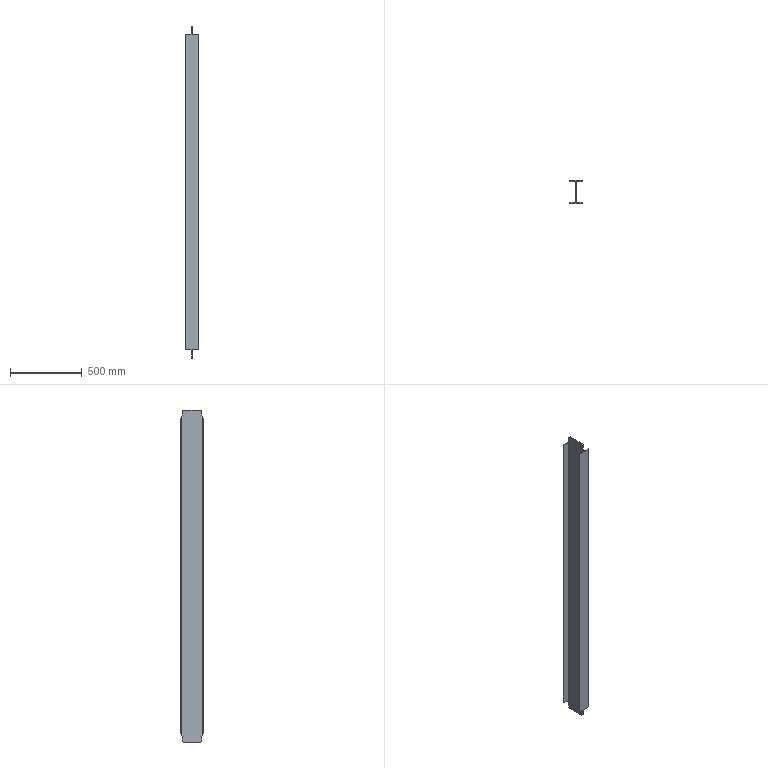Part | SolidWorks | features Chamfer 1, Extrusion 1, ICE 1 | 1 solid | 26 faces | box 88 x 160 x 2320 mm | volume 4382373 mm3 | plane 26
STEP:
#1=CARTESIAN_POINT('',(44.,-80.,1103.));
#2=VERTEX_POINT('',#1);
#3=CARTESIAN_POINT('',(44.,-80.,-1103.));
#4=VERTEX_POINT('',#3);
#5=CARTESIAN_POINT('',(44.,-80.,1160.));
#6=DIRECTION('',(0.,0.,-1.));
#7=VECTOR('',#6,1000.);
#8=LINE('',#5,#7);
#9=EDGE_CURVE('',#2,#4,#8,.T.);
#10=ORIENTED_EDGE('',*,*,#9,.F.);
#11=CARTESIAN_POINT('',(-44.,-80.,1103.));
#12=VERTEX_POINT('',#11);
#13=CARTESIAN_POINT('',(-44.,-80.,1103.));
#14=DIRECTION('',(1.,0.,0.));
#15=VECTOR('',#14,1000.);
#16=LINE('',#13,#15);
#17=EDGE_CURVE('',#12,#2,#16,.T.);
#18=ORIENTED_EDGE('',*,*,#17,.F.);
#19=CARTESIAN_POINT('',(-44.,-80.,-1103.));
#20=VERTEX_POINT('',#19);
#21=CARTESIAN_POINT('',(-44.,-80.,1160.));
#22=DIRECTION('',(0.,0.,-1.));
#23=VECTOR('',#22,1000.);
#24=LINE('',#21,#23);
#25=EDGE_CURVE('',#12,#20,#24,.T.);
#26=ORIENTED_EDGE('',*,*,#25,.T.);
#27=CARTESIAN_POINT('',(-44.,-80.,-1103.));
#28=DIRECTION('',(1.,0.,0.));
#29=VECTOR('',#28,1000.);
#30=LINE('',#27,#29);
#31=EDGE_CURVE('',#20,#4,#30,.T.);
#32=ORIENTED_EDGE('',*,*,#31,.T.);
#33=EDGE_LOOP('',(#10,#18,#26,#32));
#34=FACE_OUTER_BOUND('',#33,.T.);
#35=CARTESIAN_POINT('',(44.,-80.,1160.));
#36=DIRECTION('',(0.,1.,0.));
#37=DIRECTION('',(-1.,0.,0.));
#38=AXIS2_PLACEMENT_3D('',#35,#36,#37);
#39=PLANE('',#38);
#40=ADVANCED_FACE('',(#34),#39,.F.);
#41=CARTESIAN_POINT('',(44.,-76.,1103.));
#42=VERTEX_POINT('',#41);
#43=CARTESIAN_POINT('',(44.,-76.,-1103.));
#44=VERTEX_POINT('',#43);
#45=CARTESIAN_POINT('',(44.,-76.,1160.));
#46=DIRECTION('',(0.,0.,-1.));
#47=VECTOR('',#46,1000.);
#48=LINE('',#45,#47);
#49=EDGE_CURVE('',#42,#44,#48,.T.);
#50=ORIENTED_EDGE('',*,*,#49,.F.);
#51=CARTESIAN_POINT('',(44.,-72.,1103.));
#52=DIRECTION('',(0.,1.,0.));
#53=VECTOR('',#52,1000.);
#54=LINE('',#51,#53);
#55=EDGE_CURVE('',#2,#42,#54,.T.);
#56=ORIENTED_EDGE('',*,*,#55,.F.);
#57=ORIENTED_EDGE('',*,*,#9,.T.);
#58=CARTESIAN_POINT('',(44.,-72.,-1103.));
#59=DIRECTION('',(0.,-1.,0.));
#60=VECTOR('',#59,1000.);
#61=LINE('',#58,#60);
#62=EDGE_CURVE('',#44,#4,#61,.T.);
#63=ORIENTED_EDGE('',*,*,#62,.F.);
#64=EDGE_LOOP('',(#50,#56,#57,#63));
#65=FACE_OUTER_BOUND('',#64,.T.);
#66=CARTESIAN_POINT('',(44.,-80.,1160.));
#67=DIRECTION('',(-1.,0.,0.));
#68=DIRECTION('',(0.,-1.,0.));
#69=AXIS2_PLACEMENT_3D('',#66,#67,#68);
#70=PLANE('',#69);
#71=ADVANCED_FACE('',(#65),#70,.F.);
#72=CARTESIAN_POINT('',(3.,-72.,1103.));
#73=VERTEX_POINT('',#72);
#74=CARTESIAN_POINT('',(3.,-72.,-1103.));
#75=VERTEX_POINT('',#74);
#76=CARTESIAN_POINT('',(3.,-72.,1160.));
#77=DIRECTION('',(0.,0.,-1.));
#78=VECTOR('',#77,1000.);
#79=LINE('',#76,#78);
#80=EDGE_CURVE('',#73,#75,#79,.T.);
#81=ORIENTED_EDGE('',*,*,#80,.F.);
#82=CARTESIAN_POINT('',(44.,-76.,1103.));
#83=DIRECTION('',(0.9953,-0.0971,0.));
#84=VECTOR('',#83,1000.);
#85=LINE('',#82,#84);
#86=EDGE_CURVE('',#73,#42,#85,.T.);
#87=ORIENTED_EDGE('',*,*,#86,.T.);
#88=ORIENTED_EDGE('',*,*,#49,.T.);
#89=CARTESIAN_POINT('',(44.,-76.,-1103.));
#90=DIRECTION('',(-0.9953,0.0971,0.));
#91=VECTOR('',#90,1000.);
#92=LINE('',#89,#91);
#93=EDGE_CURVE('',#44,#75,#92,.T.);
#94=ORIENTED_EDGE('',*,*,#93,.T.);
#95=EDGE_LOOP('',(#81,#87,#88,#94));
#96=FACE_OUTER_BOUND('',#95,.T.);
#97=CARTESIAN_POINT('',(44.,-76.,1160.));
#98=DIRECTION('',(-0.0971,-0.9953,0.));
#99=DIRECTION('',(0.9953,-0.0971,0.));
#100=AXIS2_PLACEMENT_3D('',#97,#98,#99);
#101=PLANE('',#100);
#102=ADVANCED_FACE('',(#96),#101,.F.);
#103=CARTESIAN_POINT('',(3.,-66.706,-1153.294));
#104=VERTEX_POINT('',#103);
#105=CARTESIAN_POINT('',(3.,-306.022,1120.208));
#106=DIRECTION('',(0.,0.1047,-0.9945));
#107=VECTOR('',#106,1000.);
#108=LINE('',#105,#107);
#109=EDGE_CURVE('',#75,#104,#108,.T.);
#110=ORIENTED_EDGE('',*,*,#109,.T.);
#111=CARTESIAN_POINT('',(3.,-60.,-1160.));
#112=VERTEX_POINT('',#111);
#113=CARTESIAN_POINT('',(3.,-66.706,-1153.294));
#114=DIRECTION('',(0.,0.7071,-0.7071));
#115=VECTOR('',#114,1000.);
#116=LINE('',#113,#115);
#117=EDGE_CURVE('',#104,#112,#116,.T.);
#118=ORIENTED_EDGE('',*,*,#117,.T.);
#119=CARTESIAN_POINT('',(3.,60.,-1160.));
#120=VERTEX_POINT('',#119);
#121=CARTESIAN_POINT('',(3.,72.,-1160.));
#122=DIRECTION('',(0.,1.,0.));
#123=VECTOR('',#122,1000.);
#124=LINE('',#121,#123);
#125=EDGE_CURVE('',#112,#120,#124,.T.);
#126=ORIENTED_EDGE('',*,*,#125,.T.);
#127=CARTESIAN_POINT('',(3.,66.706,-1153.294));
#128=VERTEX_POINT('',#127);
#129=CARTESIAN_POINT('',(3.,66.706,-1153.294));
#130=DIRECTION('',(0.,0.7071,0.7071));
#131=VECTOR('',#130,1000.);
#132=LINE('',#129,#131);
#133=EDGE_CURVE('',#120,#128,#132,.T.);
#134=ORIENTED_EDGE('',*,*,#133,.T.);
#135=CARTESIAN_POINT('',(3.,72.,-1103.));
#136=VERTEX_POINT('',#135);
#137=CARTESIAN_POINT('',(3.,307.6,1135.2));
#138=DIRECTION('',(0.,0.1047,0.9945));
#139=VECTOR('',#138,1000.);
#140=LINE('',#137,#139);
#141=EDGE_CURVE('',#128,#136,#140,.T.);
#142=ORIENTED_EDGE('',*,*,#141,.T.);
#143=CARTESIAN_POINT('',(3.,72.,1103.));
#144=VERTEX_POINT('',#143);
#145=CARTESIAN_POINT('',(3.,72.,1160.));
#146=DIRECTION('',(0.,0.,-1.));
#147=VECTOR('',#146,1000.);
#148=LINE('',#145,#147);
#149=EDGE_CURVE('',#144,#136,#148,.T.);
#150=ORIENTED_EDGE('',*,*,#149,.F.);
#151=CARTESIAN_POINT('',(3.,66.628,1154.033));
#152=VERTEX_POINT('',#151);
#153=CARTESIAN_POINT('',(3.,66.066,1159.375));
#154=DIRECTION('',(0.,-0.1047,0.9945));
#155=VECTOR('',#154,1000.);
#156=LINE('',#153,#155);
#157=EDGE_CURVE('',#144,#152,#156,.T.);
#158=ORIENTED_EDGE('',*,*,#157,.T.);
#159=CARTESIAN_POINT('',(3.,59.257,1160.));
#160=VERTEX_POINT('',#159);
#161=CARTESIAN_POINT('',(3.,59.257,1160.));
#162=DIRECTION('',(0.,-0.7772,0.6292));
#163=VECTOR('',#162,1000.);
#164=LINE('',#161,#163);
#165=EDGE_CURVE('',#152,#160,#164,.T.);
#166=ORIENTED_EDGE('',*,*,#165,.T.);
#167=CARTESIAN_POINT('',(3.,-59.257,1160.));
#168=VERTEX_POINT('',#167);
#169=CARTESIAN_POINT('',(3.,72.,1160.));
#170=DIRECTION('',(0.,1.,0.));
#171=VECTOR('',#170,1000.);
#172=LINE('',#169,#171);
#173=EDGE_CURVE('',#168,#160,#172,.T.);
#174=ORIENTED_EDGE('',*,*,#173,.F.);
#175=CARTESIAN_POINT('',(3.,-66.628,1154.033));
#176=VERTEX_POINT('',#175);
#177=CARTESIAN_POINT('',(3.,-59.257,1160.));
#178=DIRECTION('',(0.,-0.7772,-0.6292));
#179=VECTOR('',#178,1000.);
#180=LINE('',#177,#179);
#181=EDGE_CURVE('',#168,#176,#180,.T.);
#182=ORIENTED_EDGE('',*,*,#181,.T.);
#183=CARTESIAN_POINT('',(3.,-64.488,1174.367));
#184=DIRECTION('',(0.,-0.1047,-0.9945));
#185=VECTOR('',#184,1000.);
#186=LINE('',#183,#185);
#187=EDGE_CURVE('',#176,#73,#186,.T.);
#188=ORIENTED_EDGE('',*,*,#187,.T.);
#189=ORIENTED_EDGE('',*,*,#80,.T.);
#190=EDGE_LOOP('',(#110,#118,#126,#134,#142,#150,#158,#166,#174,#182,#188,#189));
#191=FACE_OUTER_BOUND('',#190,.T.);
#192=CARTESIAN_POINT('',(3.,72.,1160.));
#193=DIRECTION('',(-1.,0.,0.));
#194=DIRECTION('',(0.,0.,1.));
#195=AXIS2_PLACEMENT_3D('',#192,#193,#194);
#196=PLANE('',#195);
#197=ADVANCED_FACE('',(#191),#196,.F.);
#198=ORIENTED_EDGE('',*,*,#149,.T.);
#199=CARTESIAN_POINT('',(44.,76.,-1103.));
#200=VERTEX_POINT('',#199);
#201=CARTESIAN_POINT('',(44.,76.,-1103.));
#202=DIRECTION('',(0.9953,0.0971,0.));
#203=VECTOR('',#202,1000.);
#204=LINE('',#201,#203);
#205=EDGE_CURVE('',#136,#200,#204,.T.);
#206=ORIENTED_EDGE('',*,*,#205,.T.);
#207=CARTESIAN_POINT('',(44.,76.,1103.));
#208=VERTEX_POINT('',#207);
#209=CARTESIAN_POINT('',(44.,76.,1160.));
#210=DIRECTION('',(0.,0.,-1.));
#211=VECTOR('',#210,1000.);
#212=LINE('',#209,#211);
#213=EDGE_CURVE('',#208,#200,#212,.T.);
#214=ORIENTED_EDGE('',*,*,#213,.F.);
#215=CARTESIAN_POINT('',(44.,76.,1103.));
#216=DIRECTION('',(-0.9953,-0.0971,0.));
#217=VECTOR('',#216,1000.);
#218=LINE('',#215,#217);
#219=EDGE_CURVE('',#208,#144,#218,.T.);
#220=ORIENTED_EDGE('',*,*,#219,.T.);
#221=EDGE_LOOP('',(#198,#206,#214,#220));
#222=FACE_OUTER_BOUND('',#221,.T.);
#223=CARTESIAN_POINT('',(44.,76.,1160.));
#224=DIRECTION('',(-0.0971,0.9953,0.));
#225=DIRECTION('',(-0.9953,-0.0971,0.));
#226=AXIS2_PLACEMENT_3D('',#223,#224,#225);
#227=PLANE('',#226);
#228=ADVANCED_FACE('',(#222),#227,.F.);
#229=ORIENTED_EDGE('',*,*,#213,.T.);
#230=CARTESIAN_POINT('',(44.,80.,-1103.));
#231=VERTEX_POINT('',#230);
#232=CARTESIAN_POINT('',(44.,72.,-1103.));
#233=DIRECTION('',(0.,-1.,0.));
#234=VECTOR('',#233,1000.);
#235=LINE('',#232,#234);
#236=EDGE_CURVE('',#231,#200,#235,.T.);
#237=ORIENTED_EDGE('',*,*,#236,.F.);
#238=CARTESIAN_POINT('',(44.,80.,1103.));
#239=VERTEX_POINT('',#238);
#240=CARTESIAN_POINT('',(44.,80.,1160.));
#241=DIRECTION('',(0.,0.,-1.));
#242=VECTOR('',#241,1000.);
#243=LINE('',#240,#242);
#244=EDGE_CURVE('',#239,#231,#243,.T.);
#245=ORIENTED_EDGE('',*,*,#244,.F.);
#246=CARTESIAN_POINT('',(44.,72.,1103.));
#247=DIRECTION('',(0.,1.,0.));
#248=VECTOR('',#247,1000.);
#249=LINE('',#246,#248);
#250=EDGE_CURVE('',#208,#239,#249,.T.);
#251=ORIENTED_EDGE('',*,*,#250,.F.);
#252=EDGE_LOOP('',(#229,#237,#245,#251));
#253=FACE_OUTER_BOUND('',#252,.T.);
#254=CARTESIAN_POINT('',(44.,80.,1160.));
#255=DIRECTION('',(-1.,0.,0.));
#256=DIRECTION('',(0.,0.,1.));
#257=AXIS2_PLACEMENT_3D('',#254,#255,#256);
#258=PLANE('',#257);
#259=ADVANCED_FACE('',(#253),#258,.F.);
#260=ORIENTED_EDGE('',*,*,#244,.T.);
#261=CARTESIAN_POINT('',(-44.,80.,-1103.));
#262=VERTEX_POINT('',#261);
#263=CARTESIAN_POINT('',(-44.,80.,-1103.));
#264=DIRECTION('',(1.,0.,0.));
#265=VECTOR('',#264,1000.);
#266=LINE('',#263,#265);
#267=EDGE_CURVE('',#262,#231,#266,.T.);
#268=ORIENTED_EDGE('',*,*,#267,.F.);
#269=CARTESIAN_POINT('',(-44.,80.,1103.));
#270=VERTEX_POINT('',#269);
#271=CARTESIAN_POINT('',(-44.,80.,1160.));
#272=DIRECTION('',(0.,0.,-1.));
#273=VECTOR('',#272,1000.);
#274=LINE('',#271,#273);
#275=EDGE_CURVE('',#270,#262,#274,.T.);
#276=ORIENTED_EDGE('',*,*,#275,.F.);
#277=CARTESIAN_POINT('',(-44.,80.,1103.));
#278=DIRECTION('',(1.,0.,0.));
#279=VECTOR('',#278,1000.);
#280=LINE('',#277,#279);
#281=EDGE_CURVE('',#270,#239,#280,.T.);
#282=ORIENTED_EDGE('',*,*,#281,.T.);
#283=EDGE_LOOP('',(#260,#268,#276,#282));
#284=FACE_OUTER_BOUND('',#283,.T.);
#285=CARTESIAN_POINT('',(44.,80.,1160.));
#286=DIRECTION('',(0.,-1.,0.));
#287=DIRECTION('',(1.,0.,0.));
#288=AXIS2_PLACEMENT_3D('',#285,#286,#287);
#289=PLANE('',#288);
#290=ADVANCED_FACE('',(#284),#289,.F.);
#291=ORIENTED_EDGE('',*,*,#275,.T.);
#292=CARTESIAN_POINT('',(-44.,76.,-1103.));
#293=VERTEX_POINT('',#292);
#294=CARTESIAN_POINT('',(-44.,72.,-1103.));
#295=DIRECTION('',(0.,-1.,0.));
#296=VECTOR('',#295,1000.);
#297=LINE('',#294,#296);
#298=EDGE_CURVE('',#262,#293,#297,.T.);
#299=ORIENTED_EDGE('',*,*,#298,.T.);
#300=CARTESIAN_POINT('',(-44.,76.,1103.));
#301=VERTEX_POINT('',#300);
#302=CARTESIAN_POINT('',(-44.,76.,1160.));
#303=DIRECTION('',(0.,0.,-1.));
#304=VECTOR('',#303,1000.);
#305=LINE('',#302,#304);
#306=EDGE_CURVE('',#301,#293,#305,.T.);
#307=ORIENTED_EDGE('',*,*,#306,.F.);
#308=CARTESIAN_POINT('',(-44.,72.,1103.));
#309=DIRECTION('',(0.,1.,0.));
#310=VECTOR('',#309,1000.);
#311=LINE('',#308,#310);
#312=EDGE_CURVE('',#301,#270,#311,.T.);
#313=ORIENTED_EDGE('',*,*,#312,.T.);
#314=EDGE_LOOP('',(#291,#299,#307,#313));
#315=FACE_OUTER_BOUND('',#314,.T.);
#316=CARTESIAN_POINT('',(-44.,80.,1160.));
#317=DIRECTION('',(1.,0.,0.));
#318=DIRECTION('',(0.,1.,0.));
#319=AXIS2_PLACEMENT_3D('',#316,#317,#318);
#320=PLANE('',#319);
#321=ADVANCED_FACE('',(#315),#320,.F.);
#322=ORIENTED_EDGE('',*,*,#306,.T.);
#323=CARTESIAN_POINT('',(-3.,72.,-1103.));
#324=VERTEX_POINT('',#323);
#325=CARTESIAN_POINT('',(-44.,76.,-1103.));
#326=DIRECTION('',(0.9953,-0.0971,0.));
#327=VECTOR('',#326,1000.);
#328=LINE('',#325,#327);
#329=EDGE_CURVE('',#293,#324,#328,.T.);
#330=ORIENTED_EDGE('',*,*,#329,.T.);
#331=CARTESIAN_POINT('',(-3.,72.,1103.));
#332=VERTEX_POINT('',#331);
#333=CARTESIAN_POINT('',(-3.,72.,1160.));
#334=DIRECTION('',(0.,0.,-1.));
#335=VECTOR('',#334,1000.);
#336=LINE('',#333,#335);
#337=EDGE_CURVE('',#332,#324,#336,.T.);
#338=ORIENTED_EDGE('',*,*,#337,.F.);
#339=CARTESIAN_POINT('',(-44.,76.,1103.));
#340=DIRECTION('',(-0.9953,0.0971,0.));
#341=VECTOR('',#340,1000.);
#342=LINE('',#339,#341);
#343=EDGE_CURVE('',#332,#301,#342,.T.);
#344=ORIENTED_EDGE('',*,*,#343,.T.);
#345=EDGE_LOOP('',(#322,#330,#338,#344));
#346=FACE_OUTER_BOUND('',#345,.T.);
#347=CARTESIAN_POINT('',(-44.,76.,1160.));
#348=DIRECTION('',(0.0971,0.9953,0.));
#349=DIRECTION('',(-0.9953,0.0971,0.));
#350=AXIS2_PLACEMENT_3D('',#347,#348,#349);
#351=PLANE('',#350);
#352=ADVANCED_FACE('',(#346),#351,.F.);
#353=CARTESIAN_POINT('',(-3.,60.,-1160.));
#354=VERTEX_POINT('',#353);
#355=CARTESIAN_POINT('',(-3.,-60.,-1160.));
#356=VERTEX_POINT('',#355);
#357=CARTESIAN_POINT('',(-3.,72.,-1160.));
#358=DIRECTION('',(0.,-1.,0.));
#359=VECTOR('',#358,1000.);
#360=LINE('',#357,#359);
#361=EDGE_CURVE('',#354,#356,#360,.T.);
#362=ORIENTED_EDGE('',*,*,#361,.T.);
#363=CARTESIAN_POINT('',(-3.,-66.706,-1153.294));
#364=VERTEX_POINT('',#363);
#365=CARTESIAN_POINT('',(-3.,-66.706,-1153.294));
#366=DIRECTION('',(0.,-0.7071,0.7071));
#367=VECTOR('',#366,1000.);
#368=LINE('',#365,#367);
#369=EDGE_CURVE('',#356,#364,#368,.T.);
#370=ORIENTED_EDGE('',*,*,#369,.T.);
#371=CARTESIAN_POINT('',(-3.,-72.,-1103.));
#372=VERTEX_POINT('',#371);
#373=CARTESIAN_POINT('',(-3.,-306.022,1120.208));
#374=DIRECTION('',(0.,-0.1047,0.9945));
#375=VECTOR('',#374,1000.);
#376=LINE('',#373,#375);
#377=EDGE_CURVE('',#364,#372,#376,.T.);
#378=ORIENTED_EDGE('',*,*,#377,.T.);
#379=CARTESIAN_POINT('',(-3.,-72.,1103.));
#380=VERTEX_POINT('',#379);
#381=CARTESIAN_POINT('',(-3.,-72.,1160.));
#382=DIRECTION('',(0.,0.,-1.));
#383=VECTOR('',#382,1000.);
#384=LINE('',#381,#383);
#385=EDGE_CURVE('',#380,#372,#384,.T.);
#386=ORIENTED_EDGE('',*,*,#385,.F.);
#387=CARTESIAN_POINT('',(-3.,-66.628,1154.033));
#388=VERTEX_POINT('',#387);
#389=CARTESIAN_POINT('',(-3.,-64.488,1174.367));
#390=DIRECTION('',(0.,0.1047,0.9945));
#391=VECTOR('',#390,1000.);
#392=LINE('',#389,#391);
#393=EDGE_CURVE('',#380,#388,#392,.T.);
#394=ORIENTED_EDGE('',*,*,#393,.T.);
#395=CARTESIAN_POINT('',(-3.,-59.257,1160.));
#396=VERTEX_POINT('',#395);
#397=CARTESIAN_POINT('',(-3.,-59.257,1160.));
#398=DIRECTION('',(0.,0.7772,0.6292));
#399=VECTOR('',#398,1000.);
#400=LINE('',#397,#399);
#401=EDGE_CURVE('',#388,#396,#400,.T.);
#402=ORIENTED_EDGE('',*,*,#401,.T.);
#403=CARTESIAN_POINT('',(-3.,59.257,1160.));
#404=VERTEX_POINT('',#403);
#405=CARTESIAN_POINT('',(-3.,72.,1160.));
#406=DIRECTION('',(0.,-1.,0.));
#407=VECTOR('',#406,1000.);
#408=LINE('',#405,#407);
#409=EDGE_CURVE('',#404,#396,#408,.T.);
#410=ORIENTED_EDGE('',*,*,#409,.F.);
#411=CARTESIAN_POINT('',(-3.,66.628,1154.033));
#412=VERTEX_POINT('',#411);
#413=CARTESIAN_POINT('',(-3.,59.257,1160.));
#414=DIRECTION('',(0.,0.7772,-0.6292));
#415=VECTOR('',#414,1000.);
#416=LINE('',#413,#415);
#417=EDGE_CURVE('',#404,#412,#416,.T.);
#418=ORIENTED_EDGE('',*,*,#417,.T.);
#419=CARTESIAN_POINT('',(-3.,66.066,1159.375));
#420=DIRECTION('',(0.,0.1047,-0.9945));
#421=VECTOR('',#420,1000.);
#422=LINE('',#419,#421);
#423=EDGE_CURVE('',#412,#332,#422,.T.);
#424=ORIENTED_EDGE('',*,*,#423,.T.);
#425=ORIENTED_EDGE('',*,*,#337,.T.);
#426=CARTESIAN_POINT('',(-3.,66.706,-1153.294));
#427=VERTEX_POINT('',#426);
#428=CARTESIAN_POINT('',(-3.,307.6,1135.2));
#429=DIRECTION('',(0.,-0.1047,-0.9945));
#430=VECTOR('',#429,1000.);
#431=LINE('',#428,#430);
#432=EDGE_CURVE('',#324,#427,#431,.T.);
#433=ORIENTED_EDGE('',*,*,#432,.T.);
#434=CARTESIAN_POINT('',(-3.,66.706,-1153.294));
#435=DIRECTION('',(0.,-0.7071,-0.7071));
#436=VECTOR('',#435,1000.);
#437=LINE('',#434,#436);
#438=EDGE_CURVE('',#427,#354,#437,.T.);
#439=ORIENTED_EDGE('',*,*,#438,.T.);
#440=EDGE_LOOP('',(#362,#370,#378,#386,#394,#402,#410,#418,#424,#425,#433,#439));
#441=FACE_OUTER_BOUND('',#440,.T.);
#442=CARTESIAN_POINT('',(-3.,72.,1160.));
#443=DIRECTION('',(1.,0.,0.));
#444=DIRECTION('',(0.,0.,-1.));
#445=AXIS2_PLACEMENT_3D('',#442,#443,#444);
#446=PLANE('',#445);
#447=ADVANCED_FACE('',(#441),#446,.F.);
#448=CARTESIAN_POINT('',(-44.,-76.,1103.));
#449=VERTEX_POINT('',#448);
#450=CARTESIAN_POINT('',(-44.,-76.,-1103.));
#451=VERTEX_POINT('',#450);
#452=CARTESIAN_POINT('',(-44.,-76.,1160.));
#453=DIRECTION('',(0.,0.,-1.));
#454=VECTOR('',#453,1000.);
#455=LINE('',#452,#454);
#456=EDGE_CURVE('',#449,#451,#455,.T.);
#457=ORIENTED_EDGE('',*,*,#456,.F.);
#458=CARTESIAN_POINT('',(-44.,-76.,1103.));
#459=DIRECTION('',(0.9953,0.0971,0.));
#460=VECTOR('',#459,1000.);
#461=LINE('',#458,#460);
#462=EDGE_CURVE('',#449,#380,#461,.T.);
#463=ORIENTED_EDGE('',*,*,#462,.T.);
#464=ORIENTED_EDGE('',*,*,#385,.T.);
#465=CARTESIAN_POINT('',(-44.,-76.,-1103.));
#466=DIRECTION('',(-0.9953,-0.0971,0.));
#467=VECTOR('',#466,1000.);
#468=LINE('',#465,#467);
#469=EDGE_CURVE('',#372,#451,#468,.T.);
#470=ORIENTED_EDGE('',*,*,#469,.T.);
#471=EDGE_LOOP('',(#457,#463,#464,#470));
#472=FACE_OUTER_BOUND('',#471,.T.);
#473=CARTESIAN_POINT('',(-44.,-76.,1160.));
#474=DIRECTION('',(0.0971,-0.9953,0.));
#475=DIRECTION('',(0.9953,0.0971,0.));
#476=AXIS2_PLACEMENT_3D('',#473,#474,#475);
#477=PLANE('',#476);
#478=ADVANCED_FACE('',(#472),#477,.F.);
#479=ORIENTED_EDGE('',*,*,#25,.F.);
#480=CARTESIAN_POINT('',(-44.,-72.,1103.));
#481=DIRECTION('',(0.,1.,0.));
#482=VECTOR('',#481,1000.);
#483=LINE('',#480,#482);
#484=EDGE_CURVE('',#12,#449,#483,.T.);
#485=ORIENTED_EDGE('',*,*,#484,.T.);
#486=ORIENTED_EDGE('',*,*,#456,.T.);
#487=CARTESIAN_POINT('',(-44.,-72.,-1103.));
#488=DIRECTION('',(0.,-1.,0.));
#489=VECTOR('',#488,1000.);
#490=LINE('',#487,#489);
#491=EDGE_CURVE('',#451,#20,#490,.T.);
#492=ORIENTED_EDGE('',*,*,#491,.T.);
#493=EDGE_LOOP('',(#479,#485,#486,#492));
#494=FACE_OUTER_BOUND('',#493,.T.);
#495=CARTESIAN_POINT('',(-44.,-80.,1160.));
#496=DIRECTION('',(1.,0.,0.));
#497=DIRECTION('',(0.,1.,0.));
#498=AXIS2_PLACEMENT_3D('',#495,#496,#497);
#499=PLANE('',#498);
#500=ADVANCED_FACE('',(#494),#499,.F.);
#501=ORIENTED_EDGE('',*,*,#409,.T.);
#502=CARTESIAN_POINT('',(0.,-59.257,1160.));
#503=DIRECTION('',(1.,0.,0.));
#504=VECTOR('',#503,1000.);
#505=LINE('',#502,#504);
#506=EDGE_CURVE('',#396,#168,#505,.T.);
#507=ORIENTED_EDGE('',*,*,#506,.T.);
#508=ORIENTED_EDGE('',*,*,#173,.T.);
#509=CARTESIAN_POINT('',(0.,59.257,1160.));
#510=DIRECTION('',(-1.,0.,0.));
#511=VECTOR('',#510,1000.);
#512=LINE('',#509,#511);
#513=EDGE_CURVE('',#160,#404,#512,.T.);
#514=ORIENTED_EDGE('',*,*,#513,.T.);
#515=EDGE_LOOP('',(#501,#507,#508,#514));
#516=FACE_OUTER_BOUND('',#515,.T.);
#517=CARTESIAN_POINT('',(0.,0.,1160.));
#518=DIRECTION('',(0.,0.,-1.));
#519=DIRECTION('',(-1.,0.,0.));
#520=AXIS2_PLACEMENT_3D('',#517,#518,#519);
#521=PLANE('',#520);
#522=ADVANCED_FACE('',(#516),#521,.F.);
#523=ORIENTED_EDGE('',*,*,#125,.F.);
#524=CARTESIAN_POINT('',(-3.,-60.,-1160.));
#525=DIRECTION('',(-1.,0.,0.));
#526=VECTOR('',#525,1000.);
#527=LINE('',#524,#526);
#528=EDGE_CURVE('',#112,#356,#527,.T.);
#529=ORIENTED_EDGE('',*,*,#528,.T.);
#530=ORIENTED_EDGE('',*,*,#361,.F.);
#531=CARTESIAN_POINT('',(3.,60.,-1160.));
#532=DIRECTION('',(1.,0.,0.));
#533=VECTOR('',#532,1000.);
#534=LINE('',#531,#533);
#535=EDGE_CURVE('',#354,#120,#534,.T.);
#536=ORIENTED_EDGE('',*,*,#535,.T.);
#537=EDGE_LOOP('',(#523,#529,#530,#536));
#538=FACE_OUTER_BOUND('',#537,.T.);
#539=CARTESIAN_POINT('',(0.,0.,-1160.));
#540=DIRECTION('',(0.,0.,-1.));
#541=DIRECTION('',(-1.,0.,0.));
#542=AXIS2_PLACEMENT_3D('',#539,#540,#541);
#543=PLANE('',#542);
#544=ADVANCED_FACE('',(#538),#543,.T.);
#545=CARTESIAN_POINT('',(-44.,72.,-1103.));
#546=DIRECTION('',(1.,0.,0.));
#547=VECTOR('',#546,1000.);
#548=LINE('',#545,#547);
#549=EDGE_CURVE('',#324,#136,#548,.T.);
#550=ORIENTED_EDGE('',*,*,#549,.F.);
#551=ORIENTED_EDGE('',*,*,#329,.F.);
#552=ORIENTED_EDGE('',*,*,#298,.F.);
#553=ORIENTED_EDGE('',*,*,#267,.T.);
#554=ORIENTED_EDGE('',*,*,#236,.T.);
#555=ORIENTED_EDGE('',*,*,#205,.F.);
#556=EDGE_LOOP('',(#550,#551,#552,#553,#554,#555));
#557=FACE_OUTER_BOUND('',#556,.T.);
#558=CARTESIAN_POINT('',(-44.,72.,-1103.));
#559=DIRECTION('',(0.,0.,1.));
#560=DIRECTION('',(1.,0.,0.));
#561=AXIS2_PLACEMENT_3D('',#558,#559,#560);
#562=PLANE('',#561);
#563=ADVANCED_FACE('',(#557),#562,.F.);
#564=ORIENTED_EDGE('',*,*,#141,.F.);
#565=CARTESIAN_POINT('',(-3.,66.706,-1153.294));
#566=DIRECTION('',(-1.,0.,0.));
#567=VECTOR('',#566,1000.);
#568=LINE('',#565,#567);
#569=EDGE_CURVE('',#128,#427,#568,.T.);
#570=ORIENTED_EDGE('',*,*,#569,.T.);
#571=ORIENTED_EDGE('',*,*,#432,.F.);
#572=ORIENTED_EDGE('',*,*,#549,.T.);
#573=EDGE_LOOP('',(#564,#570,#571,#572));
#574=FACE_OUTER_BOUND('',#573,.T.);
#575=CARTESIAN_POINT('',(-44.,66.,-1160.));
#576=DIRECTION('',(0.,-0.9945,0.1047));
#577=DIRECTION('',(0.,-0.1047,-0.9945));
#578=AXIS2_PLACEMENT_3D('',#575,#576,#577);
#579=PLANE('',#578);
#580=ADVANCED_FACE('',(#574),#579,.F.);
#581=ORIENTED_EDGE('',*,*,#62,.T.);
#582=ORIENTED_EDGE('',*,*,#31,.F.);
#583=ORIENTED_EDGE('',*,*,#491,.F.);
#584=ORIENTED_EDGE('',*,*,#469,.F.);
#585=CARTESIAN_POINT('',(-44.,-72.,-1103.));
#586=DIRECTION('',(1.,0.,0.));
#587=VECTOR('',#586,1000.);
#588=LINE('',#585,#587);
#589=EDGE_CURVE('',#372,#75,#588,.T.);
#590=ORIENTED_EDGE('',*,*,#589,.T.);
#591=ORIENTED_EDGE('',*,*,#93,.F.);
#592=EDGE_LOOP('',(#581,#582,#583,#584,#590,#591));
#593=FACE_OUTER_BOUND('',#592,.T.);
#594=CARTESIAN_POINT('',(-44.,-72.,-1103.));
#595=DIRECTION('',(0.,0.,1.));
#596=DIRECTION('',(0.,-1.,0.));
#597=AXIS2_PLACEMENT_3D('',#594,#595,#596);
#598=PLANE('',#597);
#599=ADVANCED_FACE('',(#593),#598,.F.);
#600=ORIENTED_EDGE('',*,*,#377,.F.);
#601=CARTESIAN_POINT('',(3.,-66.706,-1153.294));
#602=DIRECTION('',(1.,0.,0.));
#603=VECTOR('',#602,1000.);
#604=LINE('',#601,#603);
#605=EDGE_CURVE('',#364,#104,#604,.T.);
#606=ORIENTED_EDGE('',*,*,#605,.T.);
#607=ORIENTED_EDGE('',*,*,#109,.F.);
#608=ORIENTED_EDGE('',*,*,#589,.F.);
#609=EDGE_LOOP('',(#600,#606,#607,#608));
#610=FACE_OUTER_BOUND('',#609,.T.);
#611=CARTESIAN_POINT('',(-44.,-66.,-1160.));
#612=DIRECTION('',(0.,0.9945,0.1047));
#613=DIRECTION('',(0.,-0.1047,0.9945));
#614=AXIS2_PLACEMENT_3D('',#611,#612,#613);
#615=PLANE('',#614);
#616=ADVANCED_FACE('',(#610),#615,.F.);
#617=ORIENTED_EDGE('',*,*,#250,.T.);
#618=ORIENTED_EDGE('',*,*,#281,.F.);
#619=ORIENTED_EDGE('',*,*,#312,.F.);
#620=ORIENTED_EDGE('',*,*,#343,.F.);
#621=CARTESIAN_POINT('',(-44.,72.,1103.));
#622=DIRECTION('',(1.,0.,0.));
#623=VECTOR('',#622,1000.);
#624=LINE('',#621,#623);
#625=EDGE_CURVE('',#332,#144,#624,.T.);
#626=ORIENTED_EDGE('',*,*,#625,.T.);
#627=ORIENTED_EDGE('',*,*,#219,.F.);
#628=EDGE_LOOP('',(#617,#618,#619,#620,#626,#627));
#629=FACE_OUTER_BOUND('',#628,.T.);
#630=CARTESIAN_POINT('',(-44.,72.,1103.));
#631=DIRECTION('',(0.,0.,-1.));
#632=DIRECTION('',(-1.,0.,0.));
#633=AXIS2_PLACEMENT_3D('',#630,#631,#632);
#634=PLANE('',#633);
#635=ADVANCED_FACE('',(#629),#634,.F.);
#636=ORIENTED_EDGE('',*,*,#423,.F.);
#637=CARTESIAN_POINT('',(-44.,66.628,1154.033));
#638=DIRECTION('',(1.,0.,0.));
#639=VECTOR('',#638,1000.);
#640=LINE('',#637,#639);
#641=EDGE_CURVE('',#412,#152,#640,.T.);
#642=ORIENTED_EDGE('',*,*,#641,.T.);
#643=ORIENTED_EDGE('',*,*,#157,.F.);
#644=ORIENTED_EDGE('',*,*,#625,.F.);
#645=EDGE_LOOP('',(#636,#642,#643,#644));
#646=FACE_OUTER_BOUND('',#645,.T.);
#647=CARTESIAN_POINT('',(-44.,66.,1160.));
#648=DIRECTION('',(0.,-0.9945,-0.1047));
#649=DIRECTION('',(0.,0.1047,-0.9945));
#650=AXIS2_PLACEMENT_3D('',#647,#648,#649);
#651=PLANE('',#650);
#652=ADVANCED_FACE('',(#646),#651,.F.);
#653=CARTESIAN_POINT('',(-44.,-72.,1103.));
#654=DIRECTION('',(1.,0.,0.));
#655=VECTOR('',#654,1000.);
#656=LINE('',#653,#655);
#657=EDGE_CURVE('',#380,#73,#656,.T.);
#658=ORIENTED_EDGE('',*,*,#657,.F.);
#659=ORIENTED_EDGE('',*,*,#462,.F.);
#660=ORIENTED_EDGE('',*,*,#484,.F.);
#661=ORIENTED_EDGE('',*,*,#17,.T.);
#662=ORIENTED_EDGE('',*,*,#55,.T.);
#663=ORIENTED_EDGE('',*,*,#86,.F.);
#664=EDGE_LOOP('',(#658,#659,#660,#661,#662,#663));
#665=FACE_OUTER_BOUND('',#664,.T.);
#666=CARTESIAN_POINT('',(-44.,-72.,1103.));
#667=DIRECTION('',(0.,0.,-1.));
#668=DIRECTION('',(0.,1.,0.));
#669=AXIS2_PLACEMENT_3D('',#666,#667,#668);
#670=PLANE('',#669);
#671=ADVANCED_FACE('',(#665),#670,.F.);
#672=ORIENTED_EDGE('',*,*,#187,.F.);
#673=CARTESIAN_POINT('',(-44.,-66.628,1154.033));
#674=DIRECTION('',(-1.,0.,0.));
#675=VECTOR('',#674,1000.);
#676=LINE('',#673,#675);
#677=EDGE_CURVE('',#176,#388,#676,.T.);
#678=ORIENTED_EDGE('',*,*,#677,.T.);
#679=ORIENTED_EDGE('',*,*,#393,.F.);
#680=ORIENTED_EDGE('',*,*,#657,.T.);
#681=EDGE_LOOP('',(#672,#678,#679,#680));
#682=FACE_OUTER_BOUND('',#681,.T.);
#683=CARTESIAN_POINT('',(-44.,-66.,1160.));
#684=DIRECTION('',(0.,0.9945,-0.1047));
#685=DIRECTION('',(0.,0.1047,0.9945));
#686=AXIS2_PLACEMENT_3D('',#683,#684,#685);
#687=PLANE('',#686);
#688=ADVANCED_FACE('',(#682),#687,.F.);
#689=ORIENTED_EDGE('',*,*,#369,.F.);
#690=ORIENTED_EDGE('',*,*,#528,.F.);
#691=ORIENTED_EDGE('',*,*,#117,.F.);
#692=ORIENTED_EDGE('',*,*,#605,.F.);
#693=EDGE_LOOP('',(#689,#690,#691,#692));
#694=FACE_OUTER_BOUND('',#693,.T.);
#695=CARTESIAN_POINT('',(-44.,-66.706,-1153.294));
#696=DIRECTION('',(0.,-0.7071,-0.7071));
#697=DIRECTION('',(-1.,0.,0.));
#698=AXIS2_PLACEMENT_3D('',#695,#696,#697);
#699=PLANE('',#698);
#700=ADVANCED_FACE('',(#694),#699,.T.);
#701=ORIENTED_EDGE('',*,*,#133,.F.);
#702=ORIENTED_EDGE('',*,*,#535,.F.);
#703=ORIENTED_EDGE('',*,*,#438,.F.);
#704=ORIENTED_EDGE('',*,*,#569,.F.);
#705=EDGE_LOOP('',(#701,#702,#703,#704));
#706=FACE_OUTER_BOUND('',#705,.T.);
#707=CARTESIAN_POINT('',(-44.,66.706,-1153.294));
#708=DIRECTION('',(0.,0.7071,-0.7071));
#709=DIRECTION('',(1.,0.,0.));
#710=AXIS2_PLACEMENT_3D('',#707,#708,#709);
#711=PLANE('',#710);
#712=ADVANCED_FACE('',(#706),#711,.T.);
#713=ORIENTED_EDGE('',*,*,#401,.F.);
#714=ORIENTED_EDGE('',*,*,#677,.F.);
#715=ORIENTED_EDGE('',*,*,#181,.F.);
#716=ORIENTED_EDGE('',*,*,#506,.F.);
#717=EDGE_LOOP('',(#713,#714,#715,#716));
#718=FACE_OUTER_BOUND('',#717,.T.);
#719=CARTESIAN_POINT('',(0.,-59.257,1160.));
#720=DIRECTION('',(0.,0.6292,-0.7772));
#721=DIRECTION('',(1.,0.,0.));
#722=AXIS2_PLACEMENT_3D('',#719,#720,#721);
#723=PLANE('',#722);
#724=ADVANCED_FACE('',(#718),#723,.F.);
#725=ORIENTED_EDGE('',*,*,#165,.F.);
#726=ORIENTED_EDGE('',*,*,#641,.F.);
#727=ORIENTED_EDGE('',*,*,#417,.F.);
#728=ORIENTED_EDGE('',*,*,#513,.F.);
#729=EDGE_LOOP('',(#725,#726,#727,#728));
#730=FACE_OUTER_BOUND('',#729,.T.);
#731=CARTESIAN_POINT('',(0.,59.257,1160.));
#732=DIRECTION('',(0.,-0.6292,-0.7772));
#733=DIRECTION('',(-1.,0.,0.));
#734=AXIS2_PLACEMENT_3D('',#731,#732,#733);
#735=PLANE('',#734);
#736=ADVANCED_FACE('',(#730),#735,.F.);
#737=CLOSED_SHELL('',(#40,#71,#102,#197,#228,#259,#290,#321,#352,#447,#478,#500,#522,#544,#563,#580,#599,#616,#635,#652,#671,#688,#700,#712,#724,#736));
#738=MANIFOLD_SOLID_BREP('',#737);
#739=CARTESIAN_POINT('',(0.,0.,0.));
#740=DIRECTION('',(0.,0.,1.));
#741=DIRECTION('',(1.,0.,0.));
#742=AXIS2_PLACEMENT_3D('',#739,#740,#741);
#743=(LENGTH_UNIT()NAMED_UNIT(*)SI_UNIT(.MILLI.,.METRE.));
#744=UNCERTAINTY_MEASURE_WITH_UNIT(LENGTH_MEASURE(0.00001),#743,'','');
#745=(NAMED_UNIT(*)PLANE_ANGLE_UNIT()SI_UNIT($,.RADIAN.));
#746=(NAMED_UNIT(*)SI_UNIT($,.STERADIAN.)SOLID_ANGLE_UNIT());
#747=(GEOMETRIC_REPRESENTATION_CONTEXT(3)GLOBAL_UNCERTAINTY_ASSIGNED_CONTEXT((#744))GLOBAL_UNIT_ASSIGNED_CONTEXT((#743,#745,#746))REPRESENTATION_CONTEXT('',''));
#748=ADVANCED_BREP_SHAPE_REPRESENTATION('',(#738,#742),#747);